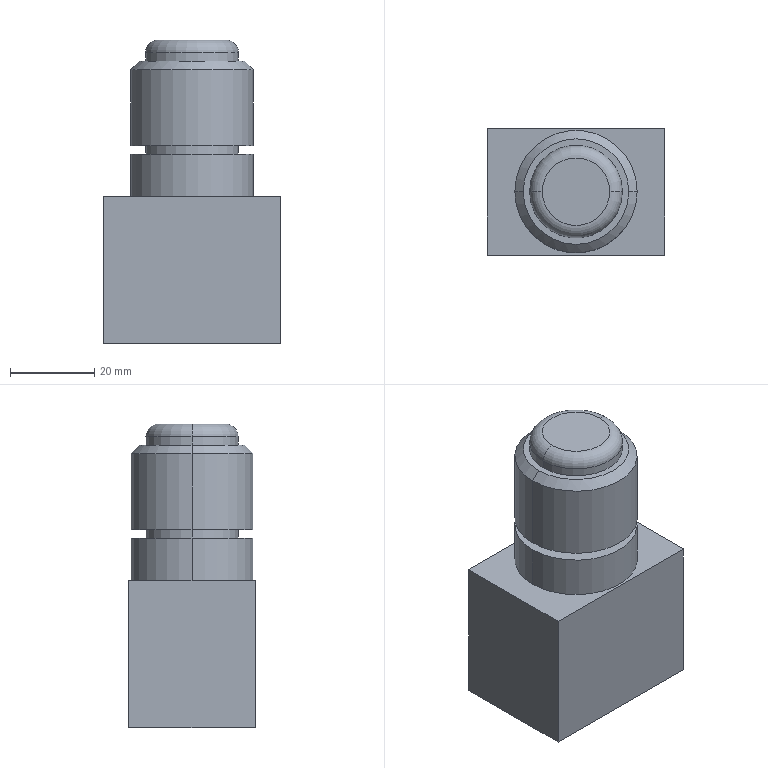Part | STEP file | Push button | 1 solid | 22 faces | box 42 x 30 x 72 mm | volume 66277 mm3 | plane 10 | cylinder 8 | cone 2 | torus 2 | commonest cylinder face diameters 22 x4 29 x4
STEP:
#1=CARTESIAN_POINT('',(0.,0.,0.));
#2=DIRECTION('',(0.,0.,1.));
#3=DIRECTION('',(1.,0.,0.));
#4=AXIS2_PLACEMENT_3D('',#1,#2,#3);
#5=CARTESIAN_POINT('',(12.5,0.,67.));
#6=VERTEX_POINT('',#5);
#7=CARTESIAN_POINT('',(-12.5,0.,67.));
#8=VERTEX_POINT('',#7);
#9=CARTESIAN_POINT('',(0.,0.,67.));
#10=DIRECTION('',(0.,0.,1.));
#11=DIRECTION('',(1.,0.,0.));
#12=AXIS2_PLACEMENT_3D('',#9,#10,#11);
#13=CIRCLE('',#12,12.5);
#14=CARTESIAN_POINT('',(0.,0.,67.));
#15=DIRECTION('',(0.,0.,-1.));
#16=DIRECTION('',(-1.,0.,0.));
#17=AXIS2_PLACEMENT_3D('',#14,#15,#16);
#18=CONICAL_SURFACE('',#17,12.5,0.7854);
#19=CARTESIAN_POINT('',(3.142,0.));
#20=DIRECTION('',(-1.,0.));
#21=VECTOR('',#20,1.);
#22=LINE('',#19,#21);
#23=(GEOMETRIC_REPRESENTATION_CONTEXT(2)PARAMETRIC_REPRESENTATION_CONTEXT()REPRESENTATION_CONTEXT('',''));
#24=DEFINITIONAL_REPRESENTATION('',(#22),#23);
#25=PCURVE('',#18,#24);
#26=CARTESIAN_POINT('',(0.,0.,67.));
#27=DIRECTION('',(0.,0.,1.));
#28=DIRECTION('',(1.,0.,0.));
#29=AXIS2_PLACEMENT_3D('',#26,#27,#28);
#30=PLANE('',#29);
#31=CARTESIAN_POINT('',(0.,0.));
#32=DIRECTION('',(1.,0.));
#33=AXIS2_PLACEMENT_2D('',#31,#32);
#34=CIRCLE('',#33,12.5);
#35=(GEOMETRIC_REPRESENTATION_CONTEXT(2)PARAMETRIC_REPRESENTATION_CONTEXT()REPRESENTATION_CONTEXT('',''));
#36=DEFINITIONAL_REPRESENTATION('',(#34),#35);
#37=PCURVE('',#30,#36);
#38=SURFACE_CURVE('',#13,(#25,#37),.PCURVE_S1.);
#39=EDGE_CURVE('',#6,#8,#38,.T.);
#40=ORIENTED_EDGE('',*,*,#39,.F.);
#41=CARTESIAN_POINT('',(14.5,0.,65.));
#42=VERTEX_POINT('',#41);
#43=CARTESIAN_POINT('',(12.5,0.,67.));
#44=DIRECTION('',(0.7071,0.,-0.7071));
#45=VECTOR('',#44,1.);
#46=LINE('',#43,#45);
#47=CARTESIAN_POINT('',(3.142,0.));
#48=DIRECTION('',(0.,1.));
#49=VECTOR('',#48,1.);
#50=LINE('',#47,#49);
#51=(GEOMETRIC_REPRESENTATION_CONTEXT(2)PARAMETRIC_REPRESENTATION_CONTEXT()REPRESENTATION_CONTEXT('',''));
#52=DEFINITIONAL_REPRESENTATION('',(#50),#51);
#53=PCURVE('',#18,#52);
#54=CARTESIAN_POINT('',(0.,0.,67.));
#55=DIRECTION('',(0.,0.,-1.));
#56=DIRECTION('',(-1.,0.,0.));
#57=AXIS2_PLACEMENT_3D('',#54,#55,#56);
#58=CONICAL_SURFACE('',#57,12.5,0.7854);
#59=CARTESIAN_POINT('',(3.142,0.));
#60=DIRECTION('',(0.,1.));
#61=VECTOR('',#60,1.);
#62=LINE('',#59,#61);
#63=(GEOMETRIC_REPRESENTATION_CONTEXT(2)PARAMETRIC_REPRESENTATION_CONTEXT()REPRESENTATION_CONTEXT('',''));
#64=DEFINITIONAL_REPRESENTATION('',(#62),#63);
#65=PCURVE('',#58,#64);
#66=SURFACE_CURVE('',#46,(#53,#65),.PCURVE_S1.);
#67=EDGE_CURVE('',#6,#42,#66,.T.);
#68=ORIENTED_EDGE('',*,*,#67,.T.);
#69=CARTESIAN_POINT('',(-14.5,0.,65.));
#70=VERTEX_POINT('',#69);
#71=CARTESIAN_POINT('',(0.,0.,65.));
#72=DIRECTION('',(0.,0.,-1.));
#73=DIRECTION('',(1.,0.,0.));
#74=AXIS2_PLACEMENT_3D('',#71,#72,#73);
#75=CIRCLE('',#74,14.5);
#76=CARTESIAN_POINT('',(-3.142,2.));
#77=DIRECTION('',(1.,0.));
#78=VECTOR('',#77,1.);
#79=LINE('',#76,#78);
#80=(GEOMETRIC_REPRESENTATION_CONTEXT(2)PARAMETRIC_REPRESENTATION_CONTEXT()REPRESENTATION_CONTEXT('',''));
#81=DEFINITIONAL_REPRESENTATION('',(#79),#80);
#82=PCURVE('',#18,#81);
#83=CARTESIAN_POINT('',(0.,0.,67.));
#84=DIRECTION('',(0.,0.,-1.));
#85=DIRECTION('',(-1.,0.,0.));
#86=AXIS2_PLACEMENT_3D('',#83,#84,#85);
#87=CYLINDRICAL_SURFACE('',#86,14.5);
#88=CARTESIAN_POINT('',(-3.142,2.));
#89=DIRECTION('',(1.,0.));
#90=VECTOR('',#89,1.);
#91=LINE('',#88,#90);
#92=(GEOMETRIC_REPRESENTATION_CONTEXT(2)PARAMETRIC_REPRESENTATION_CONTEXT()REPRESENTATION_CONTEXT('',''));
#93=DEFINITIONAL_REPRESENTATION('',(#91),#92);
#94=PCURVE('',#87,#93);
#95=SURFACE_CURVE('',#75,(#82,#94),.PCURVE_S1.);
#96=EDGE_CURVE('',#70,#42,#95,.T.);
#97=ORIENTED_EDGE('',*,*,#96,.F.);
#98=CARTESIAN_POINT('',(-12.5,0.,67.));
#99=DIRECTION('',(-0.7071,0.,-0.7071));
#100=VECTOR('',#99,1.);
#101=LINE('',#98,#100);
#102=CARTESIAN_POINT('',(0.,0.));
#103=DIRECTION('',(0.,1.));
#104=VECTOR('',#103,1.);
#105=LINE('',#102,#104);
#106=(GEOMETRIC_REPRESENTATION_CONTEXT(2)PARAMETRIC_REPRESENTATION_CONTEXT()REPRESENTATION_CONTEXT('',''));
#107=DEFINITIONAL_REPRESENTATION('',(#105),#106);
#108=PCURVE('',#18,#107);
#109=CARTESIAN_POINT('',(6.283,0.));
#110=DIRECTION('',(0.,1.));
#111=VECTOR('',#110,1.);
#112=LINE('',#109,#111);
#113=(GEOMETRIC_REPRESENTATION_CONTEXT(2)PARAMETRIC_REPRESENTATION_CONTEXT()REPRESENTATION_CONTEXT('',''));
#114=DEFINITIONAL_REPRESENTATION('',(#112),#113);
#115=PCURVE('',#58,#114);
#116=SURFACE_CURVE('',#101,(#108,#115),.PCURVE_S1.);
#117=EDGE_CURVE('',#8,#70,#116,.T.);
#118=ORIENTED_EDGE('',*,*,#117,.F.);
#119=EDGE_LOOP('',(#40,#68,#97,#118));
#120=FACE_BOUND('',#119,.T.);
#121=ADVANCED_FACE('',(#120),#18,.T.);
#122=CARTESIAN_POINT('',(-11.,0.,69.));
#123=VERTEX_POINT('',#122);
#124=CARTESIAN_POINT('',(11.,0.,69.));
#125=VERTEX_POINT('',#124);
#126=CARTESIAN_POINT('',(0.,0.,69.));
#127=DIRECTION('',(0.,0.,-1.));
#128=DIRECTION('',(1.,0.,0.));
#129=AXIS2_PLACEMENT_3D('',#126,#127,#128);
#130=CIRCLE('',#129,11.);
#131=CARTESIAN_POINT('',(0.,0.,69.));
#132=DIRECTION('',(0.,0.,1.));
#133=DIRECTION('',(1.,0.,0.));
#134=AXIS2_PLACEMENT_3D('',#131,#132,#133);
#135=TOROIDAL_SURFACE('',#134,8.,3.);
#136=CARTESIAN_POINT('',(6.283,0.));
#137=DIRECTION('',(-1.,0.));
#138=VECTOR('',#137,1.);
#139=LINE('',#136,#138);
#140=(GEOMETRIC_REPRESENTATION_CONTEXT(2)PARAMETRIC_REPRESENTATION_CONTEXT()REPRESENTATION_CONTEXT('',''));
#141=DEFINITIONAL_REPRESENTATION('',(#139),#140);
#142=PCURVE('',#135,#141);
#143=CARTESIAN_POINT('',(0.,0.,72.));
#144=DIRECTION('',(0.,0.,-1.));
#145=DIRECTION('',(-1.,0.,0.));
#146=AXIS2_PLACEMENT_3D('',#143,#144,#145);
#147=CYLINDRICAL_SURFACE('',#146,11.);
#148=CARTESIAN_POINT('',(-3.142,3.));
#149=DIRECTION('',(1.,0.));
#150=VECTOR('',#149,1.);
#151=LINE('',#148,#150);
#152=(GEOMETRIC_REPRESENTATION_CONTEXT(2)PARAMETRIC_REPRESENTATION_CONTEXT()REPRESENTATION_CONTEXT('',''));
#153=DEFINITIONAL_REPRESENTATION('',(#151),#152);
#154=PCURVE('',#147,#153);
#155=SURFACE_CURVE('',#130,(#142,#154),.PCURVE_S1.);
#156=EDGE_CURVE('',#123,#125,#155,.T.);
#157=ORIENTED_EDGE('',*,*,#156,.F.);
#158=CARTESIAN_POINT('',(-8.,0.,72.));
#159=VERTEX_POINT('',#158);
#160=CARTESIAN_POINT('',(-8.,0.,69.));
#161=DIRECTION('',(0.,1.,0.));
#162=DIRECTION('',(-1.,0.,0.));
#163=AXIS2_PLACEMENT_3D('',#160,#161,#162);
#164=CIRCLE('',#163,3.);
#165=CARTESIAN_POINT('',(3.142,0.));
#166=DIRECTION('',(0.,1.));
#167=VECTOR('',#166,1.);
#168=LINE('',#165,#167);
#169=(GEOMETRIC_REPRESENTATION_CONTEXT(2)PARAMETRIC_REPRESENTATION_CONTEXT()REPRESENTATION_CONTEXT('',''));
#170=DEFINITIONAL_REPRESENTATION('',(#168),#169);
#171=PCURVE('',#135,#170);
#172=CARTESIAN_POINT('',(0.,0.,69.));
#173=DIRECTION('',(0.,0.,1.));
#174=DIRECTION('',(1.,0.,0.));
#175=AXIS2_PLACEMENT_3D('',#172,#173,#174);
#176=TOROIDAL_SURFACE('',#175,8.,3.);
#177=CARTESIAN_POINT('',(3.142,0.));
#178=DIRECTION('',(0.,1.));
#179=VECTOR('',#178,1.);
#180=LINE('',#177,#179);
#181=(GEOMETRIC_REPRESENTATION_CONTEXT(2)PARAMETRIC_REPRESENTATION_CONTEXT()REPRESENTATION_CONTEXT('',''));
#182=DEFINITIONAL_REPRESENTATION('',(#180),#181);
#183=PCURVE('',#176,#182);
#184=SURFACE_CURVE('',#164,(#171,#183),.PCURVE_S1.);
#185=EDGE_CURVE('',#123,#159,#184,.T.);
#186=ORIENTED_EDGE('',*,*,#185,.T.);
#187=CARTESIAN_POINT('',(8.,0.,72.));
#188=VERTEX_POINT('',#187);
#189=CARTESIAN_POINT('',(0.,0.,72.));
#190=DIRECTION('',(0.,0.,1.));
#191=DIRECTION('',(1.,0.,0.));
#192=AXIS2_PLACEMENT_3D('',#189,#190,#191);
#193=CIRCLE('',#192,8.);
#194=CARTESIAN_POINT('',(0.,1.571));
#195=DIRECTION('',(1.,0.));
#196=VECTOR('',#195,1.);
#197=LINE('',#194,#196);
#198=(GEOMETRIC_REPRESENTATION_CONTEXT(2)PARAMETRIC_REPRESENTATION_CONTEXT()REPRESENTATION_CONTEXT('',''));
#199=DEFINITIONAL_REPRESENTATION('',(#197),#198);
#200=PCURVE('',#135,#199);
#201=CARTESIAN_POINT('',(0.,0.,72.));
#202=DIRECTION('',(0.,0.,1.));
#203=DIRECTION('',(1.,0.,0.));
#204=AXIS2_PLACEMENT_3D('',#201,#202,#203);
#205=PLANE('',#204);
#206=CARTESIAN_POINT('',(0.,0.));
#207=DIRECTION('',(1.,0.));
#208=AXIS2_PLACEMENT_2D('',#206,#207);
#209=CIRCLE('',#208,8.);
#210=(GEOMETRIC_REPRESENTATION_CONTEXT(2)PARAMETRIC_REPRESENTATION_CONTEXT()REPRESENTATION_CONTEXT('',''));
#211=DEFINITIONAL_REPRESENTATION('',(#209),#210);
#212=PCURVE('',#205,#211);
#213=SURFACE_CURVE('',#193,(#200,#212),.PCURVE_S1.);
#214=EDGE_CURVE('',#188,#159,#213,.T.);
#215=ORIENTED_EDGE('',*,*,#214,.F.);
#216=CARTESIAN_POINT('',(8.,0.,69.));
#217=DIRECTION('',(0.,-1.,0.));
#218=DIRECTION('',(0.,0.,-1.));
#219=AXIS2_PLACEMENT_3D('',#216,#217,#218);
#220=CIRCLE('',#219,3.);
#221=CARTESIAN_POINT('',(0.,-1.571));
#222=DIRECTION('',(0.,1.));
#223=VECTOR('',#222,1.);
#224=LINE('',#221,#223);
#225=(GEOMETRIC_REPRESENTATION_CONTEXT(2)PARAMETRIC_REPRESENTATION_CONTEXT()REPRESENTATION_CONTEXT('',''));
#226=DEFINITIONAL_REPRESENTATION('',(#224),#225);
#227=PCURVE('',#135,#226);
#228=CARTESIAN_POINT('',(6.283,-1.571));
#229=DIRECTION('',(0.,1.));
#230=VECTOR('',#229,1.);
#231=LINE('',#228,#230);
#232=(GEOMETRIC_REPRESENTATION_CONTEXT(2)PARAMETRIC_REPRESENTATION_CONTEXT()REPRESENTATION_CONTEXT('',''));
#233=DEFINITIONAL_REPRESENTATION('',(#231),#232);
#234=PCURVE('',#176,#233);
#235=SURFACE_CURVE('',#220,(#227,#234),.PCURVE_S1.);
#236=EDGE_CURVE('',#125,#188,#235,.T.);
#237=ORIENTED_EDGE('',*,*,#236,.F.);
#238=EDGE_LOOP('',(#157,#186,#215,#237));
#239=FACE_BOUND('',#238,.T.);
#240=ADVANCED_FACE('',(#239),#135,.T.);
#241=ORIENTED_EDGE('',*,*,#156,.T.);
#242=CARTESIAN_POINT('',(11.,0.,67.));
#243=VERTEX_POINT('',#242);
#244=CARTESIAN_POINT('',(11.,0.,72.));
#245=DIRECTION('',(0.,0.,-1.));
#246=VECTOR('',#245,1.);
#247=LINE('',#244,#246);
#248=CARTESIAN_POINT('',(3.142,0.));
#249=DIRECTION('',(0.,1.));
#250=VECTOR('',#249,1.);
#251=LINE('',#248,#250);
#252=(GEOMETRIC_REPRESENTATION_CONTEXT(2)PARAMETRIC_REPRESENTATION_CONTEXT()REPRESENTATION_CONTEXT('',''));
#253=DEFINITIONAL_REPRESENTATION('',(#251),#252);
#254=PCURVE('',#147,#253);
#255=CARTESIAN_POINT('',(0.,0.,72.));
#256=DIRECTION('',(0.,0.,-1.));
#257=DIRECTION('',(-1.,0.,0.));
#258=AXIS2_PLACEMENT_3D('',#255,#256,#257);
#259=CYLINDRICAL_SURFACE('',#258,11.);
#260=CARTESIAN_POINT('',(3.142,0.));
#261=DIRECTION('',(0.,1.));
#262=VECTOR('',#261,1.);
#263=LINE('',#260,#262);
#264=(GEOMETRIC_REPRESENTATION_CONTEXT(2)PARAMETRIC_REPRESENTATION_CONTEXT()REPRESENTATION_CONTEXT('',''));
#265=DEFINITIONAL_REPRESENTATION('',(#263),#264);
#266=PCURVE('',#259,#265);
#267=SURFACE_CURVE('',#247,(#254,#266),.PCURVE_S1.);
#268=EDGE_CURVE('',#125,#243,#267,.T.);
#269=ORIENTED_EDGE('',*,*,#268,.T.);
#270=CARTESIAN_POINT('',(-11.,0.,67.));
#271=VERTEX_POINT('',#270);
#272=CARTESIAN_POINT('',(0.,0.,67.));
#273=DIRECTION('',(0.,0.,1.));
#274=DIRECTION('',(1.,0.,0.));
#275=AXIS2_PLACEMENT_3D('',#272,#273,#274);
#276=CIRCLE('',#275,11.);
#277=CARTESIAN_POINT('',(3.142,5.));
#278=DIRECTION('',(-1.,0.));
#279=VECTOR('',#278,1.);
#280=LINE('',#277,#279);
#281=(GEOMETRIC_REPRESENTATION_CONTEXT(2)PARAMETRIC_REPRESENTATION_CONTEXT()REPRESENTATION_CONTEXT('',''));
#282=DEFINITIONAL_REPRESENTATION('',(#280),#281);
#283=PCURVE('',#147,#282);
#284=CARTESIAN_POINT('',(0.,0.));
#285=DIRECTION('',(1.,0.));
#286=AXIS2_PLACEMENT_2D('',#284,#285);
#287=CIRCLE('',#286,11.);
#288=(GEOMETRIC_REPRESENTATION_CONTEXT(2)PARAMETRIC_REPRESENTATION_CONTEXT()REPRESENTATION_CONTEXT('',''));
#289=DEFINITIONAL_REPRESENTATION('',(#287),#288);
#290=PCURVE('',#30,#289);
#291=SURFACE_CURVE('',#276,(#283,#290),.PCURVE_S1.);
#292=EDGE_CURVE('',#243,#271,#291,.T.);
#293=ORIENTED_EDGE('',*,*,#292,.T.);
#294=CARTESIAN_POINT('',(-11.,0.,72.));
#295=DIRECTION('',(0.,0.,-1.));
#296=VECTOR('',#295,1.);
#297=LINE('',#294,#296);
#298=CARTESIAN_POINT('',(0.,0.));
#299=DIRECTION('',(0.,1.));
#300=VECTOR('',#299,1.);
#301=LINE('',#298,#300);
#302=(GEOMETRIC_REPRESENTATION_CONTEXT(2)PARAMETRIC_REPRESENTATION_CONTEXT()REPRESENTATION_CONTEXT('',''));
#303=DEFINITIONAL_REPRESENTATION('',(#301),#302);
#304=PCURVE('',#147,#303);
#305=CARTESIAN_POINT('',(6.283,0.));
#306=DIRECTION('',(0.,1.));
#307=VECTOR('',#306,1.);
#308=LINE('',#305,#307);
#309=(GEOMETRIC_REPRESENTATION_CONTEXT(2)PARAMETRIC_REPRESENTATION_CONTEXT()REPRESENTATION_CONTEXT('',''));
#310=DEFINITIONAL_REPRESENTATION('',(#308),#309);
#311=PCURVE('',#259,#310);
#312=SURFACE_CURVE('',#297,(#304,#311),.PCURVE_S1.);
#313=EDGE_CURVE('',#123,#271,#312,.T.);
#314=ORIENTED_EDGE('',*,*,#313,.F.);
#315=EDGE_LOOP('',(#241,#269,#293,#314));
#316=FACE_BOUND('',#315,.T.);
#317=ADVANCED_FACE('',(#316),#147,.T.);
#318=ORIENTED_EDGE('',*,*,#96,.T.);
#319=CARTESIAN_POINT('',(14.5,0.,47.));
#320=VERTEX_POINT('',#319);
#321=CARTESIAN_POINT('',(14.5,0.,67.));
#322=DIRECTION('',(0.,0.,-1.));
#323=VECTOR('',#322,1.);
#324=LINE('',#321,#323);
#325=CARTESIAN_POINT('',(3.142,0.));
#326=DIRECTION('',(0.,1.));
#327=VECTOR('',#326,1.);
#328=LINE('',#325,#327);
#329=(GEOMETRIC_REPRESENTATION_CONTEXT(2)PARAMETRIC_REPRESENTATION_CONTEXT()REPRESENTATION_CONTEXT('',''));
#330=DEFINITIONAL_REPRESENTATION('',(#328),#329);
#331=PCURVE('',#87,#330);
#332=CARTESIAN_POINT('',(0.,0.,67.));
#333=DIRECTION('',(0.,0.,-1.));
#334=DIRECTION('',(-1.,0.,0.));
#335=AXIS2_PLACEMENT_3D('',#332,#333,#334);
#336=CYLINDRICAL_SURFACE('',#335,14.5);
#337=CARTESIAN_POINT('',(3.142,0.));
#338=DIRECTION('',(0.,1.));
#339=VECTOR('',#338,1.);
#340=LINE('',#337,#339);
#341=(GEOMETRIC_REPRESENTATION_CONTEXT(2)PARAMETRIC_REPRESENTATION_CONTEXT()REPRESENTATION_CONTEXT('',''));
#342=DEFINITIONAL_REPRESENTATION('',(#340),#341);
#343=PCURVE('',#336,#342);
#344=SURFACE_CURVE('',#324,(#331,#343),.PCURVE_S1.);
#345=EDGE_CURVE('',#42,#320,#344,.T.);
#346=ORIENTED_EDGE('',*,*,#345,.T.);
#347=CARTESIAN_POINT('',(-14.5,0.,47.));
#348=VERTEX_POINT('',#347);
#349=CARTESIAN_POINT('',(0.,0.,47.));
#350=DIRECTION('',(0.,0.,1.));
#351=DIRECTION('',(1.,0.,0.));
#352=AXIS2_PLACEMENT_3D('',#349,#350,#351);
#353=CIRCLE('',#352,14.5);
#354=CARTESIAN_POINT('',(3.142,20.));
#355=DIRECTION('',(-1.,0.));
#356=VECTOR('',#355,1.);
#357=LINE('',#354,#356);
#358=(GEOMETRIC_REPRESENTATION_CONTEXT(2)PARAMETRIC_REPRESENTATION_CONTEXT()REPRESENTATION_CONTEXT('',''));
#359=DEFINITIONAL_REPRESENTATION('',(#357),#358);
#360=PCURVE('',#87,#359);
#361=CARTESIAN_POINT('',(0.,0.,47.));
#362=DIRECTION('',(0.,0.,1.));
#363=DIRECTION('',(1.,0.,0.));
#364=AXIS2_PLACEMENT_3D('',#361,#362,#363);
#365=PLANE('',#364);
#366=CARTESIAN_POINT('',(0.,0.));
#367=DIRECTION('',(1.,0.));
#368=AXIS2_PLACEMENT_2D('',#366,#367);
#369=CIRCLE('',#368,14.5);
#370=(GEOMETRIC_REPRESENTATION_CONTEXT(2)PARAMETRIC_REPRESENTATION_CONTEXT()REPRESENTATION_CONTEXT('',''));
#371=DEFINITIONAL_REPRESENTATION('',(#369),#370);
#372=PCURVE('',#365,#371);
#373=SURFACE_CURVE('',#353,(#360,#372),.PCURVE_S1.);
#374=EDGE_CURVE('',#320,#348,#373,.T.);
#375=ORIENTED_EDGE('',*,*,#374,.T.);
#376=CARTESIAN_POINT('',(-14.5,0.,67.));
#377=DIRECTION('',(0.,0.,-1.));
#378=VECTOR('',#377,1.);
#379=LINE('',#376,#378);
#380=CARTESIAN_POINT('',(0.,0.));
#381=DIRECTION('',(0.,1.));
#382=VECTOR('',#381,1.);
#383=LINE('',#380,#382);
#384=(GEOMETRIC_REPRESENTATION_CONTEXT(2)PARAMETRIC_REPRESENTATION_CONTEXT()REPRESENTATION_CONTEXT('',''));
#385=DEFINITIONAL_REPRESENTATION('',(#383),#384);
#386=PCURVE('',#87,#385);
#387=CARTESIAN_POINT('',(6.283,0.));
#388=DIRECTION('',(0.,1.));
#389=VECTOR('',#388,1.);
#390=LINE('',#387,#389);
#391=(GEOMETRIC_REPRESENTATION_CONTEXT(2)PARAMETRIC_REPRESENTATION_CONTEXT()REPRESENTATION_CONTEXT('',''));
#392=DEFINITIONAL_REPRESENTATION('',(#390),#391);
#393=PCURVE('',#336,#392);
#394=SURFACE_CURVE('',#379,(#386,#393),.PCURVE_S1.);
#395=EDGE_CURVE('',#70,#348,#394,.T.);
#396=ORIENTED_EDGE('',*,*,#395,.F.);
#397=EDGE_LOOP('',(#318,#346,#375,#396));
#398=FACE_BOUND('',#397,.T.);
#399=ADVANCED_FACE('',(#398),#87,.T.);
#400=CARTESIAN_POINT('',(11.,0.,47.));
#401=VERTEX_POINT('',#400);
#402=CARTESIAN_POINT('',(-11.,0.,47.));
#403=VERTEX_POINT('',#402);
#404=CARTESIAN_POINT('',(0.,0.,47.));
#405=DIRECTION('',(0.,0.,1.));
#406=DIRECTION('',(1.,0.,0.));
#407=AXIS2_PLACEMENT_3D('',#404,#405,#406);
#408=CIRCLE('',#407,11.);
#409=CARTESIAN_POINT('',(0.,0.,47.));
#410=DIRECTION('',(0.,0.,-1.));
#411=DIRECTION('',(-1.,0.,0.));
#412=AXIS2_PLACEMENT_3D('',#409,#410,#411);
#413=CYLINDRICAL_SURFACE('',#412,11.);
#414=CARTESIAN_POINT('',(3.142,0.));
#415=DIRECTION('',(-1.,0.));
#416=VECTOR('',#415,1.);
#417=LINE('',#414,#416);
#418=(GEOMETRIC_REPRESENTATION_CONTEXT(2)PARAMETRIC_REPRESENTATION_CONTEXT()REPRESENTATION_CONTEXT('',''));
#419=DEFINITIONAL_REPRESENTATION('',(#417),#418);
#420=PCURVE('',#413,#419);
#421=CARTESIAN_POINT('',(0.,0.));
#422=DIRECTION('',(1.,0.));
#423=AXIS2_PLACEMENT_2D('',#421,#422);
#424=CIRCLE('',#423,11.);
#425=(GEOMETRIC_REPRESENTATION_CONTEXT(2)PARAMETRIC_REPRESENTATION_CONTEXT()REPRESENTATION_CONTEXT('',''));
#426=DEFINITIONAL_REPRESENTATION('',(#424),#425);
#427=PCURVE('',#365,#426);
#428=SURFACE_CURVE('',#408,(#420,#427),.PCURVE_S1.);
#429=EDGE_CURVE('',#401,#403,#428,.T.);
#430=ORIENTED_EDGE('',*,*,#429,.F.);
#431=CARTESIAN_POINT('',(11.,0.,45.));
#432=VERTEX_POINT('',#431);
#433=CARTESIAN_POINT('',(11.,0.,47.));
#434=DIRECTION('',(0.,0.,-1.));
#435=VECTOR('',#434,1.);
#436=LINE('',#433,#435);
#437=CARTESIAN_POINT('',(3.142,0.));
#438=DIRECTION('',(0.,1.));
#439=VECTOR('',#438,1.);
#440=LINE('',#437,#439);
#441=(GEOMETRIC_REPRESENTATION_CONTEXT(2)PARAMETRIC_REPRESENTATION_CONTEXT()REPRESENTATION_CONTEXT('',''));
#442=DEFINITIONAL_REPRESENTATION('',(#440),#441);
#443=PCURVE('',#413,#442);
#444=CARTESIAN_POINT('',(0.,0.,47.));
#445=DIRECTION('',(0.,0.,-1.));
#446=DIRECTION('',(-1.,0.,0.));
#447=AXIS2_PLACEMENT_3D('',#444,#445,#446);
#448=CYLINDRICAL_SURFACE('',#447,11.);
#449=CARTESIAN_POINT('',(3.142,0.));
#450=DIRECTION('',(0.,1.));
#451=VECTOR('',#450,1.);
#452=LINE('',#449,#451);
#453=(GEOMETRIC_REPRESENTATION_CONTEXT(2)PARAMETRIC_REPRESENTATION_CONTEXT()REPRESENTATION_CONTEXT('',''));
#454=DEFINITIONAL_REPRESENTATION('',(#452),#453);
#455=PCURVE('',#448,#454);
#456=SURFACE_CURVE('',#436,(#443,#455),.PCURVE_S1.);
#457=EDGE_CURVE('',#401,#432,#456,.T.);
#458=ORIENTED_EDGE('',*,*,#457,.T.);
#459=CARTESIAN_POINT('',(-11.,0.,45.));
#460=VERTEX_POINT('',#459);
#461=CARTESIAN_POINT('',(0.,0.,45.));
#462=DIRECTION('',(0.,0.,1.));
#463=DIRECTION('',(1.,0.,0.));
#464=AXIS2_PLACEMENT_3D('',#461,#462,#463);
#465=CIRCLE('',#464,11.);
#466=CARTESIAN_POINT('',(3.142,2.));
#467=DIRECTION('',(-1.,0.));
#468=VECTOR('',#467,1.);
#469=LINE('',#466,#468);
#470=(GEOMETRIC_REPRESENTATION_CONTEXT(2)PARAMETRIC_REPRESENTATION_CONTEXT()REPRESENTATION_CONTEXT('',''));
#471=DEFINITIONAL_REPRESENTATION('',(#469),#470);
#472=PCURVE('',#413,#471);
#473=CARTESIAN_POINT('',(0.,0.,45.));
#474=DIRECTION('',(0.,0.,1.));
#475=DIRECTION('',(1.,0.,0.));
#476=AXIS2_PLACEMENT_3D('',#473,#474,#475);
#477=PLANE('',#476);
#478=CARTESIAN_POINT('',(0.,0.));
#479=DIRECTION('',(1.,0.));
#480=AXIS2_PLACEMENT_2D('',#478,#479);
#481=CIRCLE('',#480,11.);
#482=(GEOMETRIC_REPRESENTATION_CONTEXT(2)PARAMETRIC_REPRESENTATION_CONTEXT()REPRESENTATION_CONTEXT('',''));
#483=DEFINITIONAL_REPRESENTATION('',(#481),#482);
#484=PCURVE('',#477,#483);
#485=SURFACE_CURVE('',#465,(#472,#484),.PCURVE_S1.);
#486=EDGE_CURVE('',#432,#460,#485,.T.);
#487=ORIENTED_EDGE('',*,*,#486,.T.);
#488=CARTESIAN_POINT('',(-11.,0.,47.));
#489=DIRECTION('',(0.,0.,-1.));
#490=VECTOR('',#489,1.);
#491=LINE('',#488,#490);
#492=CARTESIAN_POINT('',(0.,0.));
#493=DIRECTION('',(0.,1.));
#494=VECTOR('',#493,1.);
#495=LINE('',#492,#494);
#496=(GEOMETRIC_REPRESENTATION_CONTEXT(2)PARAMETRIC_REPRESENTATION_CONTEXT()REPRESENTATION_CONTEXT('',''));
#497=DEFINITIONAL_REPRESENTATION('',(#495),#496);
#498=PCURVE('',#413,#497);
#499=CARTESIAN_POINT('',(6.283,0.));
#500=DIRECTION('',(0.,1.));
#501=VECTOR('',#500,1.);
#502=LINE('',#499,#501);
#503=(GEOMETRIC_REPRESENTATION_CONTEXT(2)PARAMETRIC_REPRESENTATION_CONTEXT()REPRESENTATION_CONTEXT('',''));
#504=DEFINITIONAL_REPRESENTATION('',(#502),#503);
#505=PCURVE('',#448,#504);
#506=SURFACE_CURVE('',#491,(#498,#505),.PCURVE_S1.);
#507=EDGE_CURVE('',#403,#460,#506,.T.);
#508=ORIENTED_EDGE('',*,*,#507,.F.);
#509=EDGE_LOOP('',(#430,#458,#487,#508));
#510=FACE_BOUND('',#509,.T.);
#511=ADVANCED_FACE('',(#510),#413,.T.);
#512=CARTESIAN_POINT('',(14.5,0.,45.));
#513=VERTEX_POINT('',#512);
#514=CARTESIAN_POINT('',(-14.5,0.,45.));
#515=VERTEX_POINT('',#514);
#516=CARTESIAN_POINT('',(0.,0.,45.));
#517=DIRECTION('',(0.,0.,1.));
#518=DIRECTION('',(1.,0.,0.));
#519=AXIS2_PLACEMENT_3D('',#516,#517,#518);
#520=CIRCLE('',#519,14.5);
#521=CARTESIAN_POINT('',(0.,0.,45.));
#522=DIRECTION('',(0.,0.,-1.));
#523=DIRECTION('',(-1.,0.,0.));
#524=AXIS2_PLACEMENT_3D('',#521,#522,#523);
#525=CYLINDRICAL_SURFACE('',#524,14.5);
#526=CARTESIAN_POINT('',(3.142,0.));
#527=DIRECTION('',(-1.,0.));
#528=VECTOR('',#527,1.);
#529=LINE('',#526,#528);
#530=(GEOMETRIC_REPRESENTATION_CONTEXT(2)PARAMETRIC_REPRESENTATION_CONTEXT()REPRESENTATION_CONTEXT('',''));
#531=DEFINITIONAL_REPRESENTATION('',(#529),#530);
#532=PCURVE('',#525,#531);
#533=CARTESIAN_POINT('',(0.,0.));
#534=DIRECTION('',(1.,0.));
#535=AXIS2_PLACEMENT_2D('',#533,#534);
#536=CIRCLE('',#535,14.5);
#537=(GEOMETRIC_REPRESENTATION_CONTEXT(2)PARAMETRIC_REPRESENTATION_CONTEXT()REPRESENTATION_CONTEXT('',''));
#538=DEFINITIONAL_REPRESENTATION('',(#536),#537);
#539=PCURVE('',#477,#538);
#540=SURFACE_CURVE('',#520,(#532,#539),.PCURVE_S1.);
#541=EDGE_CURVE('',#513,#515,#540,.T.);
#542=ORIENTED_EDGE('',*,*,#541,.F.);
#543=CARTESIAN_POINT('',(14.5,0.,35.));
#544=VERTEX_POINT('',#543);
#545=CARTESIAN_POINT('',(14.5,0.,45.));
#546=DIRECTION('',(0.,0.,-1.));
#547=VECTOR('',#546,1.);
#548=LINE('',#545,#547);
#549=CARTESIAN_POINT('',(3.142,0.));
#550=DIRECTION('',(0.,1.));
#551=VECTOR('',#550,1.);
#552=LINE('',#549,#551);
#553=(GEOMETRIC_REPRESENTATION_CONTEXT(2)PARAMETRIC_REPRESENTATION_CONTEXT()REPRESENTATION_CONTEXT('',''));
#554=DEFINITIONAL_REPRESENTATION('',(#552),#553);
#555=PCURVE('',#525,#554);
#556=CARTESIAN_POINT('',(0.,0.,45.));
#557=DIRECTION('',(0.,0.,-1.));
#558=DIRECTION('',(-1.,0.,0.));
#559=AXIS2_PLACEMENT_3D('',#556,#557,#558);
#560=CYLINDRICAL_SURFACE('',#559,14.5);
#561=CARTESIAN_POINT('',(3.142,0.));
#562=DIRECTION('',(0.,1.));
#563=VECTOR('',#562,1.);
#564=LINE('',#561,#563);
#565=(GEOMETRIC_REPRESENTATION_CONTEXT(2)PARAMETRIC_REPRESENTATION_CONTEXT()REPRESENTATION_CONTEXT('',''));
#566=DEFINITIONAL_REPRESENTATION('',(#564),#565);
#567=PCURVE('',#560,#566);
#568=SURFACE_CURVE('',#548,(#555,#567),.PCURVE_S1.);
#569=EDGE_CURVE('',#513,#544,#568,.T.);
#570=ORIENTED_EDGE('',*,*,#569,.T.);
#571=CARTESIAN_POINT('',(-14.5,0.,35.));
#572=VERTEX_POINT('',#571);
#573=CARTESIAN_POINT('',(0.,0.,35.));
#574=DIRECTION('',(0.,0.,1.));
#575=DIRECTION('',(1.,0.,0.));
#576=AXIS2_PLACEMENT_3D('',#573,#574,#575);
#577=CIRCLE('',#576,14.5);
#578=CARTESIAN_POINT('',(3.142,10.));
#579=DIRECTION('',(-1.,0.));
#580=VECTOR('',#579,1.);
#581=LINE('',#578,#580);
#582=(GEOMETRIC_REPRESENTATION_CONTEXT(2)PARAMETRIC_REPRESENTATION_CONTEXT()REPRESENTATION_CONTEXT('',''));
#583=DEFINITIONAL_REPRESENTATION('',(#581),#582);
#584=PCURVE('',#525,#583);
#585=CARTESIAN_POINT('',(0.,0.,35.));
#586=DIRECTION('',(0.,0.,1.));
#587=DIRECTION('',(1.,0.,0.));
#588=AXIS2_PLACEMENT_3D('',#585,#586,#587);
#589=PLANE('',#588);
#590=CARTESIAN_POINT('',(0.,0.));
#591=DIRECTION('',(1.,0.));
#592=AXIS2_PLACEMENT_2D('',#590,#591);
#593=CIRCLE('',#592,14.5);
#594=(GEOMETRIC_REPRESENTATION_CONTEXT(2)PARAMETRIC_REPRESENTATION_CONTEXT()REPRESENTATION_CONTEXT('',''));
#595=DEFINITIONAL_REPRESENTATION('',(#593),#594);
#596=PCURVE('',#589,#595);
#597=SURFACE_CURVE('',#577,(#584,#596),.PCURVE_S1.);
#598=EDGE_CURVE('',#544,#572,#597,.T.);
#599=ORIENTED_EDGE('',*,*,#598,.T.);
#600=CARTESIAN_POINT('',(-14.5,0.,45.));
#601=DIRECTION('',(0.,0.,-1.));
#602=VECTOR('',#601,1.);
#603=LINE('',#600,#602);
#604=CARTESIAN_POINT('',(0.,0.));
#605=DIRECTION('',(0.,1.));
#606=VECTOR('',#605,1.);
#607=LINE('',#604,#606);
#608=(GEOMETRIC_REPRESENTATION_CONTEXT(2)PARAMETRIC_REPRESENTATION_CONTEXT()REPRESENTATION_CONTEXT('',''));
#609=DEFINITIONAL_REPRESENTATION('',(#607),#608);
#610=PCURVE('',#525,#609);
#611=CARTESIAN_POINT('',(6.283,0.));
#612=DIRECTION('',(0.,1.));
#613=VECTOR('',#612,1.);
#614=LINE('',#611,#613);
#615=(GEOMETRIC_REPRESENTATION_CONTEXT(2)PARAMETRIC_REPRESENTATION_CONTEXT()REPRESENTATION_CONTEXT('',''));
#616=DEFINITIONAL_REPRESENTATION('',(#614),#615);
#617=PCURVE('',#560,#616);
#618=SURFACE_CURVE('',#603,(#610,#617),.PCURVE_S1.);
#619=EDGE_CURVE('',#515,#572,#618,.T.);
#620=ORIENTED_EDGE('',*,*,#619,.F.);
#621=EDGE_LOOP('',(#542,#570,#599,#620));
#622=FACE_BOUND('',#621,.T.);
#623=ADVANCED_FACE('',(#622),#525,.T.);
#624=CARTESIAN_POINT('',(0.,0.,67.));
#625=DIRECTION('',(0.,0.,1.));
#626=DIRECTION('',(1.,0.,0.));
#627=AXIS2_PLACEMENT_3D('',#624,#625,#626);
#628=CIRCLE('',#627,12.5);
#629=CARTESIAN_POINT('',(0.,0.));
#630=DIRECTION('',(1.,0.));
#631=AXIS2_PLACEMENT_2D('',#629,#630);
#632=CIRCLE('',#631,12.5);
#633=(GEOMETRIC_REPRESENTATION_CONTEXT(2)PARAMETRIC_REPRESENTATION_CONTEXT()REPRESENTATION_CONTEXT('',''));
#634=DEFINITIONAL_REPRESENTATION('',(#632),#633);
#635=PCURVE('',#30,#634);
#636=CARTESIAN_POINT('',(9.425,0.));
#637=DIRECTION('',(-1.,0.));
#638=VECTOR('',#637,1.);
#639=LINE('',#636,#638);
#640=(GEOMETRIC_REPRESENTATION_CONTEXT(2)PARAMETRIC_REPRESENTATION_CONTEXT()REPRESENTATION_CONTEXT('',''));
#641=DEFINITIONAL_REPRESENTATION('',(#639),#640);
#642=PCURVE('',#58,#641);
#643=SURFACE_CURVE('',#628,(#635,#642),.PCURVE_S1.);
#644=EDGE_CURVE('',#8,#6,#643,.T.);
#645=ORIENTED_EDGE('',*,*,#644,.T.);
#646=ORIENTED_EDGE('',*,*,#39,.T.);
#647=EDGE_LOOP('',(#645,#646));
#648=FACE_BOUND('',#647,.T.);
#649=CARTESIAN_POINT('',(0.,0.,67.));
#650=DIRECTION('',(0.,0.,1.));
#651=DIRECTION('',(1.,0.,0.));
#652=AXIS2_PLACEMENT_3D('',#649,#650,#651);
#653=CIRCLE('',#652,11.);
#654=CARTESIAN_POINT('',(0.,0.));
#655=DIRECTION('',(1.,0.));
#656=AXIS2_PLACEMENT_2D('',#654,#655);
#657=CIRCLE('',#656,11.);
#658=(GEOMETRIC_REPRESENTATION_CONTEXT(2)PARAMETRIC_REPRESENTATION_CONTEXT()REPRESENTATION_CONTEXT('',''));
#659=DEFINITIONAL_REPRESENTATION('',(#657),#658);
#660=PCURVE('',#30,#659);
#661=CARTESIAN_POINT('',(9.425,5.));
#662=DIRECTION('',(-1.,0.));
#663=VECTOR('',#662,1.);
#664=LINE('',#661,#663);
#665=(GEOMETRIC_REPRESENTATION_CONTEXT(2)PARAMETRIC_REPRESENTATION_CONTEXT()REPRESENTATION_CONTEXT('',''));
#666=DEFINITIONAL_REPRESENTATION('',(#664),#665);
#667=PCURVE('',#259,#666);
#668=SURFACE_CURVE('',#653,(#660,#667),.PCURVE_S1.);
#669=EDGE_CURVE('',#271,#243,#668,.T.);
#670=ORIENTED_EDGE('',*,*,#669,.F.);
#671=ORIENTED_EDGE('',*,*,#292,.F.);
#672=EDGE_LOOP('',(#670,#671));
#673=FACE_BOUND('',#672,.T.);
#674=ADVANCED_FACE('',(#648,#673),#30,.T.);
#675=CARTESIAN_POINT('',(0.,0.,45.));
#676=DIRECTION('',(0.,0.,1.));
#677=DIRECTION('',(1.,0.,0.));
#678=AXIS2_PLACEMENT_3D('',#675,#676,#677);
#679=CIRCLE('',#678,14.5);
#680=CARTESIAN_POINT('',(0.,0.));
#681=DIRECTION('',(1.,0.));
#682=AXIS2_PLACEMENT_2D('',#680,#681);
#683=CIRCLE('',#682,14.5);
#684=(GEOMETRIC_REPRESENTATION_CONTEXT(2)PARAMETRIC_REPRESENTATION_CONTEXT()REPRESENTATION_CONTEXT('',''));
#685=DEFINITIONAL_REPRESENTATION('',(#683),#684);
#686=PCURVE('',#477,#685);
#687=CARTESIAN_POINT('',(9.425,0.));
#688=DIRECTION('',(-1.,0.));
#689=VECTOR('',#688,1.);
#690=LINE('',#687,#689);
#691=(GEOMETRIC_REPRESENTATION_CONTEXT(2)PARAMETRIC_REPRESENTATION_CONTEXT()REPRESENTATION_CONTEXT('',''));
#692=DEFINITIONAL_REPRESENTATION('',(#690),#691);
#693=PCURVE('',#560,#692);
#694=SURFACE_CURVE('',#679,(#686,#693),.PCURVE_S1.);
#695=EDGE_CURVE('',#515,#513,#694,.T.);
#696=ORIENTED_EDGE('',*,*,#695,.T.);
#697=ORIENTED_EDGE('',*,*,#541,.T.);
#698=EDGE_LOOP('',(#696,#697));
#699=FACE_BOUND('',#698,.T.);
#700=CARTESIAN_POINT('',(0.,0.,45.));
#701=DIRECTION('',(0.,0.,1.));
#702=DIRECTION('',(1.,0.,0.));
#703=AXIS2_PLACEMENT_3D('',#700,#701,#702);
#704=CIRCLE('',#703,11.);
#705=CARTESIAN_POINT('',(0.,0.));
#706=DIRECTION('',(1.,0.));
#707=AXIS2_PLACEMENT_2D('',#705,#706);
#708=CIRCLE('',#707,11.);
#709=(GEOMETRIC_REPRESENTATION_CONTEXT(2)PARAMETRIC_REPRESENTATION_CONTEXT()REPRESENTATION_CONTEXT('',''));
#710=DEFINITIONAL_REPRESENTATION('',(#708),#709);
#711=PCURVE('',#477,#710);
#712=CARTESIAN_POINT('',(9.425,2.));
#713=DIRECTION('',(-1.,0.));
#714=VECTOR('',#713,1.);
#715=LINE('',#712,#714);
#716=(GEOMETRIC_REPRESENTATION_CONTEXT(2)PARAMETRIC_REPRESENTATION_CONTEXT()REPRESENTATION_CONTEXT('',''));
#717=DEFINITIONAL_REPRESENTATION('',(#715),#716);
#718=PCURVE('',#448,#717);
#719=SURFACE_CURVE('',#704,(#711,#718),.PCURVE_S1.);
#720=EDGE_CURVE('',#460,#432,#719,.T.);
#721=ORIENTED_EDGE('',*,*,#720,.F.);
#722=ORIENTED_EDGE('',*,*,#486,.F.);
#723=EDGE_LOOP('',(#721,#722));
#724=FACE_BOUND('',#723,.T.);
#725=ADVANCED_FACE('',(#699,#724),#477,.T.);
#726=CARTESIAN_POINT('',(21.,-15.,35.));
#727=VERTEX_POINT('',#726);
#728=CARTESIAN_POINT('',(21.,15.,35.));
#729=VERTEX_POINT('',#728);
#730=CARTESIAN_POINT('',(21.,15.,35.));
#731=DIRECTION('',(0.,1.,0.));
#732=VECTOR('',#731,1.);
#733=LINE('',#730,#732);
#734=CARTESIAN_POINT('',(21.,15.));
#735=DIRECTION('',(0.,1.));
#736=VECTOR('',#735,1.);
#737=LINE('',#734,#736);
#738=(GEOMETRIC_REPRESENTATION_CONTEXT(2)PARAMETRIC_REPRESENTATION_CONTEXT()REPRESENTATION_CONTEXT('',''));
#739=DEFINITIONAL_REPRESENTATION('',(#737),#738);
#740=PCURVE('',#589,#739);
#741=CARTESIAN_POINT('',(21.,15.,35.));
#742=DIRECTION('',(-1.,0.,0.));
#743=DIRECTION('',(0.,-1.,0.));
#744=AXIS2_PLACEMENT_3D('',#741,#742,#743);
#745=PLANE('',#744);
#746=CARTESIAN_POINT('',(0.,0.));
#747=DIRECTION('',(-1.,0.));
#748=VECTOR('',#747,1.);
#749=LINE('',#746,#748);
#750=(GEOMETRIC_REPRESENTATION_CONTEXT(2)PARAMETRIC_REPRESENTATION_CONTEXT()REPRESENTATION_CONTEXT('',''));
#751=DEFINITIONAL_REPRESENTATION('',(#749),#750);
#752=PCURVE('',#745,#751);
#753=SURFACE_CURVE('',#733,(#740,#752),.PCURVE_S1.);
#754=EDGE_CURVE('',#727,#729,#753,.T.);
#755=ORIENTED_EDGE('',*,*,#754,.T.);
#756=CARTESIAN_POINT('',(-21.,15.,35.));
#757=VERTEX_POINT('',#756);
#758=CARTESIAN_POINT('',(-21.,15.,35.));
#759=DIRECTION('',(-1.,0.,0.));
#760=VECTOR('',#759,1.);
#761=LINE('',#758,#760);
#762=CARTESIAN_POINT('',(-21.,15.));
#763=DIRECTION('',(-1.,0.));
#764=VECTOR('',#763,1.);
#765=LINE('',#762,#764);
#766=(GEOMETRIC_REPRESENTATION_CONTEXT(2)PARAMETRIC_REPRESENTATION_CONTEXT()REPRESENTATION_CONTEXT('',''));
#767=DEFINITIONAL_REPRESENTATION('',(#765),#766);
#768=PCURVE('',#589,#767);
#769=CARTESIAN_POINT('',(-21.,15.,35.));
#770=DIRECTION('',(0.,-1.,0.));
#771=DIRECTION('',(0.,0.,-1.));
#772=AXIS2_PLACEMENT_3D('',#769,#770,#771);
#773=PLANE('',#772);
#774=CARTESIAN_POINT('',(0.,0.));
#775=DIRECTION('',(0.,-1.));
#776=VECTOR('',#775,1.);
#777=LINE('',#774,#776);
#778=(GEOMETRIC_REPRESENTATION_CONTEXT(2)PARAMETRIC_REPRESENTATION_CONTEXT()REPRESENTATION_CONTEXT('',''));
#779=DEFINITIONAL_REPRESENTATION('',(#777),#778);
#780=PCURVE('',#773,#779);
#781=SURFACE_CURVE('',#761,(#768,#780),.PCURVE_S1.);
#782=EDGE_CURVE('',#729,#757,#781,.T.);
#783=ORIENTED_EDGE('',*,*,#782,.T.);
#784=CARTESIAN_POINT('',(-21.,-15.,35.));
#785=VERTEX_POINT('',#784);
#786=CARTESIAN_POINT('',(-21.,15.,35.));
#787=DIRECTION('',(0.,-1.,0.));
#788=VECTOR('',#787,1.);
#789=LINE('',#786,#788);
#790=CARTESIAN_POINT('',(-21.,15.));
#791=DIRECTION('',(0.,-1.));
#792=VECTOR('',#791,1.);
#793=LINE('',#790,#792);
#794=(GEOMETRIC_REPRESENTATION_CONTEXT(2)PARAMETRIC_REPRESENTATION_CONTEXT()REPRESENTATION_CONTEXT('',''));
#795=DEFINITIONAL_REPRESENTATION('',(#793),#794);
#796=PCURVE('',#589,#795);
#797=CARTESIAN_POINT('',(-21.,15.,35.));
#798=DIRECTION('',(1.,0.,0.));
#799=DIRECTION('',(0.,0.,-1.));
#800=AXIS2_PLACEMENT_3D('',#797,#798,#799);
#801=PLANE('',#800);
#802=CARTESIAN_POINT('',(0.,0.));
#803=DIRECTION('',(0.,-1.));
#804=VECTOR('',#803,1.);
#805=LINE('',#802,#804);
#806=(GEOMETRIC_REPRESENTATION_CONTEXT(2)PARAMETRIC_REPRESENTATION_CONTEXT()REPRESENTATION_CONTEXT('',''));
#807=DEFINITIONAL_REPRESENTATION('',(#805),#806);
#808=PCURVE('',#801,#807);
#809=SURFACE_CURVE('',#789,(#796,#808),.PCURVE_S1.);
#810=EDGE_CURVE('',#757,#785,#809,.T.);
#811=ORIENTED_EDGE('',*,*,#810,.T.);
#812=CARTESIAN_POINT('',(-21.,-15.,35.));
#813=DIRECTION('',(1.,0.,0.));
#814=VECTOR('',#813,1.);
#815=LINE('',#812,#814);
#816=CARTESIAN_POINT('',(-21.,-15.));
#817=DIRECTION('',(1.,0.));
#818=VECTOR('',#817,1.);
#819=LINE('',#816,#818);
#820=(GEOMETRIC_REPRESENTATION_CONTEXT(2)PARAMETRIC_REPRESENTATION_CONTEXT()REPRESENTATION_CONTEXT('',''));
#821=DEFINITIONAL_REPRESENTATION('',(#819),#820);
#822=PCURVE('',#589,#821);
#823=CARTESIAN_POINT('',(-21.,-15.,35.));
#824=DIRECTION('',(0.,1.,0.));
#825=DIRECTION('',(0.,0.,1.));
#826=AXIS2_PLACEMENT_3D('',#823,#824,#825);
#827=PLANE('',#826);
#828=CARTESIAN_POINT('',(0.,0.));
#829=DIRECTION('',(0.,1.));
#830=VECTOR('',#829,1.);
#831=LINE('',#828,#830);
#832=(GEOMETRIC_REPRESENTATION_CONTEXT(2)PARAMETRIC_REPRESENTATION_CONTEXT()REPRESENTATION_CONTEXT('',''));
#833=DEFINITIONAL_REPRESENTATION('',(#831),#832);
#834=PCURVE('',#827,#833);
#835=SURFACE_CURVE('',#815,(#822,#834),.PCURVE_S1.);
#836=EDGE_CURVE('',#785,#727,#835,.T.);
#837=ORIENTED_EDGE('',*,*,#836,.T.);
#838=EDGE_LOOP('',(#755,#783,#811,#837));
#839=FACE_BOUND('',#838,.T.);
#840=CARTESIAN_POINT('',(0.,0.,35.));
#841=DIRECTION('',(0.,0.,1.));
#842=DIRECTION('',(1.,0.,0.));
#843=AXIS2_PLACEMENT_3D('',#840,#841,#842);
#844=CIRCLE('',#843,14.5);
#845=CARTESIAN_POINT('',(0.,0.));
#846=DIRECTION('',(1.,0.));
#847=AXIS2_PLACEMENT_2D('',#845,#846);
#848=CIRCLE('',#847,14.5);
#849=(GEOMETRIC_REPRESENTATION_CONTEXT(2)PARAMETRIC_REPRESENTATION_CONTEXT()REPRESENTATION_CONTEXT('',''));
#850=DEFINITIONAL_REPRESENTATION('',(#848),#849);
#851=PCURVE('',#589,#850);
#852=CARTESIAN_POINT('',(9.425,10.));
#853=DIRECTION('',(-1.,0.));
#854=VECTOR('',#853,1.);
#855=LINE('',#852,#854);
#856=(GEOMETRIC_REPRESENTATION_CONTEXT(2)PARAMETRIC_REPRESENTATION_CONTEXT()REPRESENTATION_CONTEXT('',''));
#857=DEFINITIONAL_REPRESENTATION('',(#855),#856);
#858=PCURVE('',#560,#857);
#859=SURFACE_CURVE('',#844,(#851,#858),.PCURVE_S1.);
#860=EDGE_CURVE('',#572,#544,#859,.T.);
#861=ORIENTED_EDGE('',*,*,#860,.F.);
#862=ORIENTED_EDGE('',*,*,#598,.F.);
#863=EDGE_LOOP('',(#861,#862));
#864=FACE_BOUND('',#863,.T.);
#865=ADVANCED_FACE('',(#839,#864),#589,.T.);
#866=CARTESIAN_POINT('',(21.,-15.,0.));
#867=VERTEX_POINT('',#866);
#868=CARTESIAN_POINT('',(21.,15.,0.));
#869=VERTEX_POINT('',#868);
#870=CARTESIAN_POINT('',(21.,15.,0.));
#871=DIRECTION('',(0.,1.,0.));
#872=VECTOR('',#871,1.);
#873=LINE('',#870,#872);
#874=CARTESIAN_POINT('',(0.,-35.));
#875=DIRECTION('',(-1.,0.));
#876=VECTOR('',#875,1.);
#877=LINE('',#874,#876);
#878=(GEOMETRIC_REPRESENTATION_CONTEXT(2)PARAMETRIC_REPRESENTATION_CONTEXT()REPRESENTATION_CONTEXT('',''));
#879=DEFINITIONAL_REPRESENTATION('',(#877),#878);
#880=PCURVE('',#745,#879);
#881=CARTESIAN_POINT('',(0.,0.,0.));
#882=DIRECTION('',(0.,0.,1.));
#883=DIRECTION('',(1.,0.,0.));
#884=AXIS2_PLACEMENT_3D('',#881,#882,#883);
#885=PLANE('',#884);
#886=CARTESIAN_POINT('',(21.,15.));
#887=DIRECTION('',(0.,1.));
#888=VECTOR('',#887,1.);
#889=LINE('',#886,#888);
#890=(GEOMETRIC_REPRESENTATION_CONTEXT(2)PARAMETRIC_REPRESENTATION_CONTEXT()REPRESENTATION_CONTEXT('',''));
#891=DEFINITIONAL_REPRESENTATION('',(#889),#890);
#892=PCURVE('',#885,#891);
#893=SURFACE_CURVE('',#873,(#880,#892),.PCURVE_S1.);
#894=EDGE_CURVE('',#867,#869,#893,.T.);
#895=ORIENTED_EDGE('',*,*,#894,.T.);
#896=CARTESIAN_POINT('',(21.,15.,35.));
#897=DIRECTION('',(0.,0.,-1.));
#898=VECTOR('',#897,1.);
#899=LINE('',#896,#898);
#900=CARTESIAN_POINT('',(0.,0.));
#901=DIRECTION('',(0.,-1.));
#902=VECTOR('',#901,1.);
#903=LINE('',#900,#902);
#904=(GEOMETRIC_REPRESENTATION_CONTEXT(2)PARAMETRIC_REPRESENTATION_CONTEXT()REPRESENTATION_CONTEXT('',''));
#905=DEFINITIONAL_REPRESENTATION('',(#903),#904);
#906=PCURVE('',#745,#905);
#907=CARTESIAN_POINT('',(0.,42.));
#908=DIRECTION('',(1.,0.));
#909=VECTOR('',#908,1.);
#910=LINE('',#907,#909);
#911=(GEOMETRIC_REPRESENTATION_CONTEXT(2)PARAMETRIC_REPRESENTATION_CONTEXT()REPRESENTATION_CONTEXT('',''));
#912=DEFINITIONAL_REPRESENTATION('',(#910),#911);
#913=PCURVE('',#773,#912);
#914=SURFACE_CURVE('',#899,(#906,#913),.PCURVE_S1.);
#915=EDGE_CURVE('',#729,#869,#914,.T.);
#916=ORIENTED_EDGE('',*,*,#915,.F.);
#917=ORIENTED_EDGE('',*,*,#754,.F.);
#918=CARTESIAN_POINT('',(21.,-15.,35.));
#919=DIRECTION('',(0.,0.,-1.));
#920=VECTOR('',#919,1.);
#921=LINE('',#918,#920);
#922=CARTESIAN_POINT('',(30.,0.));
#923=DIRECTION('',(0.,-1.));
#924=VECTOR('',#923,1.);
#925=LINE('',#922,#924);
#926=(GEOMETRIC_REPRESENTATION_CONTEXT(2)PARAMETRIC_REPRESENTATION_CONTEXT()REPRESENTATION_CONTEXT('',''));
#927=DEFINITIONAL_REPRESENTATION('',(#925),#926);
#928=PCURVE('',#745,#927);
#929=CARTESIAN_POINT('',(0.,42.));
#930=DIRECTION('',(-1.,0.));
#931=VECTOR('',#930,1.);
#932=LINE('',#929,#931);
#933=(GEOMETRIC_REPRESENTATION_CONTEXT(2)PARAMETRIC_REPRESENTATION_CONTEXT()REPRESENTATION_CONTEXT('',''));
#934=DEFINITIONAL_REPRESENTATION('',(#932),#933);
#935=PCURVE('',#827,#934);
#936=SURFACE_CURVE('',#921,(#928,#935),.PCURVE_S1.);
#937=EDGE_CURVE('',#727,#867,#936,.T.);
#938=ORIENTED_EDGE('',*,*,#937,.T.);
#939=EDGE_LOOP('',(#895,#916,#917,#938));
#940=FACE_BOUND('',#939,.T.);
#941=ADVANCED_FACE('',(#940),#745,.F.);
#942=CARTESIAN_POINT('',(-21.,15.,0.));
#943=VERTEX_POINT('',#942);
#944=CARTESIAN_POINT('',(-21.,15.,0.));
#945=DIRECTION('',(-1.,0.,0.));
#946=VECTOR('',#945,1.);
#947=LINE('',#944,#946);
#948=CARTESIAN_POINT('',(35.,0.));
#949=DIRECTION('',(0.,-1.));
#950=VECTOR('',#949,1.);
#951=LINE('',#948,#950);
#952=(GEOMETRIC_REPRESENTATION_CONTEXT(2)PARAMETRIC_REPRESENTATION_CONTEXT()REPRESENTATION_CONTEXT('',''));
#953=DEFINITIONAL_REPRESENTATION('',(#951),#952);
#954=PCURVE('',#773,#953);
#955=CARTESIAN_POINT('',(-21.,15.));
#956=DIRECTION('',(-1.,0.));
#957=VECTOR('',#956,1.);
#958=LINE('',#955,#957);
#959=(GEOMETRIC_REPRESENTATION_CONTEXT(2)PARAMETRIC_REPRESENTATION_CONTEXT()REPRESENTATION_CONTEXT('',''));
#960=DEFINITIONAL_REPRESENTATION('',(#958),#959);
#961=PCURVE('',#885,#960);
#962=SURFACE_CURVE('',#947,(#954,#961),.PCURVE_S1.);
#963=EDGE_CURVE('',#869,#943,#962,.T.);
#964=ORIENTED_EDGE('',*,*,#963,.T.);
#965=CARTESIAN_POINT('',(-21.,15.,35.));
#966=DIRECTION('',(0.,0.,-1.));
#967=VECTOR('',#966,1.);
#968=LINE('',#965,#967);
#969=CARTESIAN_POINT('',(0.,0.));
#970=DIRECTION('',(1.,0.));
#971=VECTOR('',#970,1.);
#972=LINE('',#969,#971);
#973=(GEOMETRIC_REPRESENTATION_CONTEXT(2)PARAMETRIC_REPRESENTATION_CONTEXT()REPRESENTATION_CONTEXT('',''));
#974=DEFINITIONAL_REPRESENTATION('',(#972),#973);
#975=PCURVE('',#773,#974);
#976=CARTESIAN_POINT('',(0.,0.));
#977=DIRECTION('',(1.,0.));
#978=VECTOR('',#977,1.);
#979=LINE('',#976,#978);
#980=(GEOMETRIC_REPRESENTATION_CONTEXT(2)PARAMETRIC_REPRESENTATION_CONTEXT()REPRESENTATION_CONTEXT('',''));
#981=DEFINITIONAL_REPRESENTATION('',(#979),#980);
#982=PCURVE('',#801,#981);
#983=SURFACE_CURVE('',#968,(#975,#982),.PCURVE_S1.);
#984=EDGE_CURVE('',#757,#943,#983,.T.);
#985=ORIENTED_EDGE('',*,*,#984,.F.);
#986=ORIENTED_EDGE('',*,*,#782,.F.);
#987=ORIENTED_EDGE('',*,*,#915,.T.);
#988=EDGE_LOOP('',(#964,#985,#986,#987));
#989=FACE_BOUND('',#988,.T.);
#990=ADVANCED_FACE('',(#989),#773,.F.);
#991=CARTESIAN_POINT('',(-21.,-15.,0.));
#992=VERTEX_POINT('',#991);
#993=CARTESIAN_POINT('',(-21.,15.,0.));
#994=DIRECTION('',(0.,-1.,0.));
#995=VECTOR('',#994,1.);
#996=LINE('',#993,#995);
#997=CARTESIAN_POINT('',(35.,0.));
#998=DIRECTION('',(0.,-1.));
#999=VECTOR('',#998,1.);
#1000=LINE('',#997,#999);
#1001=(GEOMETRIC_REPRESENTATION_CONTEXT(2)PARAMETRIC_REPRESENTATION_CONTEXT()REPRESENTATION_CONTEXT('',''));
#1002=DEFINITIONAL_REPRESENTATION('',(#1000),#1001);
#1003=PCURVE('',#801,#1002);
#1004=CARTESIAN_POINT('',(-21.,15.));
#1005=DIRECTION('',(0.,-1.));
#1006=VECTOR('',#1005,1.);
#1007=LINE('',#1004,#1006);
#1008=(GEOMETRIC_REPRESENTATION_CONTEXT(2)PARAMETRIC_REPRESENTATION_CONTEXT()REPRESENTATION_CONTEXT('',''));
#1009=DEFINITIONAL_REPRESENTATION('',(#1007),#1008);
#1010=PCURVE('',#885,#1009);
#1011=SURFACE_CURVE('',#996,(#1003,#1010),.PCURVE_S1.);
#1012=EDGE_CURVE('',#943,#992,#1011,.T.);
#1013=ORIENTED_EDGE('',*,*,#1012,.T.);
#1014=CARTESIAN_POINT('',(-21.,-15.,35.));
#1015=DIRECTION('',(0.,0.,-1.));
#1016=VECTOR('',#1015,1.);
#1017=LINE('',#1014,#1016);
#1018=CARTESIAN_POINT('',(0.,-30.));
#1019=DIRECTION('',(1.,0.));
#1020=VECTOR('',#1019,1.);
#1021=LINE('',#1018,#1020);
#1022=(GEOMETRIC_REPRESENTATION_CONTEXT(2)PARAMETRIC_REPRESENTATION_CONTEXT()REPRESENTATION_CONTEXT('',''));
#1023=DEFINITIONAL_REPRESENTATION('',(#1021),#1022);
#1024=PCURVE('',#801,#1023);
#1025=CARTESIAN_POINT('',(0.,0.));
#1026=DIRECTION('',(-1.,0.));
#1027=VECTOR('',#1026,1.);
#1028=LINE('',#1025,#1027);
#1029=(GEOMETRIC_REPRESENTATION_CONTEXT(2)PARAMETRIC_REPRESENTATION_CONTEXT()REPRESENTATION_CONTEXT('',''));
#1030=DEFINITIONAL_REPRESENTATION('',(#1028),#1029);
#1031=PCURVE('',#827,#1030);
#1032=SURFACE_CURVE('',#1017,(#1024,#1031),.PCURVE_S1.);
#1033=EDGE_CURVE('',#785,#992,#1032,.T.);
#1034=ORIENTED_EDGE('',*,*,#1033,.F.);
#1035=ORIENTED_EDGE('',*,*,#810,.F.);
#1036=ORIENTED_EDGE('',*,*,#984,.T.);
#1037=EDGE_LOOP('',(#1013,#1034,#1035,#1036));
#1038=FACE_BOUND('',#1037,.T.);
#1039=ADVANCED_FACE('',(#1038),#801,.F.);
#1040=CARTESIAN_POINT('',(-21.,-15.,0.));
#1041=DIRECTION('',(1.,0.,0.));
#1042=VECTOR('',#1041,1.);
#1043=LINE('',#1040,#1042);
#1044=CARTESIAN_POINT('',(-35.,0.));
#1045=DIRECTION('',(0.,1.));
#1046=VECTOR('',#1045,1.);
#1047=LINE('',#1044,#1046);
#1048=(GEOMETRIC_REPRESENTATION_CONTEXT(2)PARAMETRIC_REPRESENTATION_CONTEXT()REPRESENTATION_CONTEXT('',''));
#1049=DEFINITIONAL_REPRESENTATION('',(#1047),#1048);
#1050=PCURVE('',#827,#1049);
#1051=CARTESIAN_POINT('',(-21.,-15.));
#1052=DIRECTION('',(1.,0.));
#1053=VECTOR('',#1052,1.);
#1054=LINE('',#1051,#1053);
#1055=(GEOMETRIC_REPRESENTATION_CONTEXT(2)PARAMETRIC_REPRESENTATION_CONTEXT()REPRESENTATION_CONTEXT('',''));
#1056=DEFINITIONAL_REPRESENTATION('',(#1054),#1055);
#1057=PCURVE('',#885,#1056);
#1058=SURFACE_CURVE('',#1043,(#1050,#1057),.PCURVE_S1.);
#1059=EDGE_CURVE('',#992,#867,#1058,.T.);
#1060=ORIENTED_EDGE('',*,*,#1059,.T.);
#1061=ORIENTED_EDGE('',*,*,#937,.F.);
#1062=ORIENTED_EDGE('',*,*,#836,.F.);
#1063=ORIENTED_EDGE('',*,*,#1033,.T.);
#1064=EDGE_LOOP('',(#1060,#1061,#1062,#1063));
#1065=FACE_BOUND('',#1064,.T.);
#1066=ADVANCED_FACE('',(#1065),#827,.F.);
#1067=ORIENTED_EDGE('',*,*,#894,.F.);
#1068=ORIENTED_EDGE('',*,*,#1059,.F.);
#1069=ORIENTED_EDGE('',*,*,#1012,.F.);
#1070=ORIENTED_EDGE('',*,*,#963,.F.);
#1071=EDGE_LOOP('',(#1067,#1068,#1069,#1070));
#1072=FACE_BOUND('',#1071,.T.);
#1073=ADVANCED_FACE('',(#1072),#885,.F.);
#1074=ORIENTED_EDGE('',*,*,#569,.F.);
#1075=ORIENTED_EDGE('',*,*,#695,.F.);
#1076=ORIENTED_EDGE('',*,*,#619,.T.);
#1077=ORIENTED_EDGE('',*,*,#860,.T.);
#1078=EDGE_LOOP('',(#1074,#1075,#1076,#1077));
#1079=FACE_BOUND('',#1078,.T.);
#1080=ADVANCED_FACE('',(#1079),#560,.T.);
#1081=ORIENTED_EDGE('',*,*,#457,.F.);
#1082=CARTESIAN_POINT('',(0.,0.,47.));
#1083=DIRECTION('',(0.,0.,1.));
#1084=DIRECTION('',(1.,0.,0.));
#1085=AXIS2_PLACEMENT_3D('',#1082,#1083,#1084);
#1086=CIRCLE('',#1085,11.);
#1087=CARTESIAN_POINT('',(9.425,0.));
#1088=DIRECTION('',(-1.,0.));
#1089=VECTOR('',#1088,1.);
#1090=LINE('',#1087,#1089);
#1091=(GEOMETRIC_REPRESENTATION_CONTEXT(2)PARAMETRIC_REPRESENTATION_CONTEXT()REPRESENTATION_CONTEXT('',''));
#1092=DEFINITIONAL_REPRESENTATION('',(#1090),#1091);
#1093=PCURVE('',#448,#1092);
#1094=CARTESIAN_POINT('',(0.,0.));
#1095=DIRECTION('',(1.,0.));
#1096=AXIS2_PLACEMENT_2D('',#1094,#1095);
#1097=CIRCLE('',#1096,11.);
#1098=(GEOMETRIC_REPRESENTATION_CONTEXT(2)PARAMETRIC_REPRESENTATION_CONTEXT()REPRESENTATION_CONTEXT('',''));
#1099=DEFINITIONAL_REPRESENTATION('',(#1097),#1098);
#1100=PCURVE('',#365,#1099);
#1101=SURFACE_CURVE('',#1086,(#1093,#1100),.PCURVE_S1.);
#1102=EDGE_CURVE('',#403,#401,#1101,.T.);
#1103=ORIENTED_EDGE('',*,*,#1102,.F.);
#1104=ORIENTED_EDGE('',*,*,#507,.T.);
#1105=ORIENTED_EDGE('',*,*,#720,.T.);
#1106=EDGE_LOOP('',(#1081,#1103,#1104,#1105));
#1107=FACE_BOUND('',#1106,.T.);
#1108=ADVANCED_FACE('',(#1107),#448,.T.);
#1109=CARTESIAN_POINT('',(0.,0.,47.));
#1110=DIRECTION('',(0.,0.,1.));
#1111=DIRECTION('',(1.,0.,0.));
#1112=AXIS2_PLACEMENT_3D('',#1109,#1110,#1111);
#1113=CIRCLE('',#1112,14.5);
#1114=CARTESIAN_POINT('',(0.,0.));
#1115=DIRECTION('',(1.,0.));
#1116=AXIS2_PLACEMENT_2D('',#1114,#1115);
#1117=CIRCLE('',#1116,14.5);
#1118=(GEOMETRIC_REPRESENTATION_CONTEXT(2)PARAMETRIC_REPRESENTATION_CONTEXT()REPRESENTATION_CONTEXT('',''));
#1119=DEFINITIONAL_REPRESENTATION('',(#1117),#1118);
#1120=PCURVE('',#365,#1119);
#1121=CARTESIAN_POINT('',(9.425,20.));
#1122=DIRECTION('',(-1.,0.));
#1123=VECTOR('',#1122,1.);
#1124=LINE('',#1121,#1123);
#1125=(GEOMETRIC_REPRESENTATION_CONTEXT(2)PARAMETRIC_REPRESENTATION_CONTEXT()REPRESENTATION_CONTEXT('',''));
#1126=DEFINITIONAL_REPRESENTATION('',(#1124),#1125);
#1127=PCURVE('',#336,#1126);
#1128=SURFACE_CURVE('',#1113,(#1120,#1127),.PCURVE_S1.);
#1129=EDGE_CURVE('',#348,#320,#1128,.T.);
#1130=ORIENTED_EDGE('',*,*,#1129,.F.);
#1131=ORIENTED_EDGE('',*,*,#374,.F.);
#1132=EDGE_LOOP('',(#1130,#1131));
#1133=FACE_BOUND('',#1132,.T.);
#1134=ORIENTED_EDGE('',*,*,#1102,.T.);
#1135=ORIENTED_EDGE('',*,*,#429,.T.);
#1136=EDGE_LOOP('',(#1134,#1135));
#1137=FACE_BOUND('',#1136,.T.);
#1138=ADVANCED_FACE('',(#1133,#1137),#365,.F.);
#1139=ORIENTED_EDGE('',*,*,#345,.F.);
#1140=CARTESIAN_POINT('',(0.,0.,65.));
#1141=DIRECTION('',(0.,0.,-1.));
#1142=DIRECTION('',(1.,0.,0.));
#1143=AXIS2_PLACEMENT_3D('',#1140,#1141,#1142);
#1144=CIRCLE('',#1143,14.5);
#1145=CARTESIAN_POINT('',(3.142,2.));
#1146=DIRECTION('',(1.,0.));
#1147=VECTOR('',#1146,1.);
#1148=LINE('',#1145,#1147);
#1149=(GEOMETRIC_REPRESENTATION_CONTEXT(2)PARAMETRIC_REPRESENTATION_CONTEXT()REPRESENTATION_CONTEXT('',''));
#1150=DEFINITIONAL_REPRESENTATION('',(#1148),#1149);
#1151=PCURVE('',#336,#1150);
#1152=CARTESIAN_POINT('',(3.142,2.));
#1153=DIRECTION('',(1.,0.));
#1154=VECTOR('',#1153,1.);
#1155=LINE('',#1152,#1154);
#1156=(GEOMETRIC_REPRESENTATION_CONTEXT(2)PARAMETRIC_REPRESENTATION_CONTEXT()REPRESENTATION_CONTEXT('',''));
#1157=DEFINITIONAL_REPRESENTATION('',(#1155),#1156);
#1158=PCURVE('',#58,#1157);
#1159=SURFACE_CURVE('',#1144,(#1151,#1158),.PCURVE_S1.);
#1160=EDGE_CURVE('',#42,#70,#1159,.T.);
#1161=ORIENTED_EDGE('',*,*,#1160,.T.);
#1162=ORIENTED_EDGE('',*,*,#395,.T.);
#1163=ORIENTED_EDGE('',*,*,#1129,.T.);
#1164=EDGE_LOOP('',(#1139,#1161,#1162,#1163));
#1165=FACE_BOUND('',#1164,.T.);
#1166=ADVANCED_FACE('',(#1165),#336,.T.);
#1167=ORIENTED_EDGE('',*,*,#268,.F.);
#1168=CARTESIAN_POINT('',(0.,0.,69.));
#1169=DIRECTION('',(0.,0.,-1.));
#1170=DIRECTION('',(1.,0.,0.));
#1171=AXIS2_PLACEMENT_3D('',#1168,#1169,#1170);
#1172=CIRCLE('',#1171,11.);
#1173=CARTESIAN_POINT('',(3.142,3.));
#1174=DIRECTION('',(1.,0.));
#1175=VECTOR('',#1174,1.);
#1176=LINE('',#1173,#1175);
#1177=(GEOMETRIC_REPRESENTATION_CONTEXT(2)PARAMETRIC_REPRESENTATION_CONTEXT()REPRESENTATION_CONTEXT('',''));
#1178=DEFINITIONAL_REPRESENTATION('',(#1176),#1177);
#1179=PCURVE('',#259,#1178);
#1180=CARTESIAN_POINT('',(6.283,0.));
#1181=DIRECTION('',(-1.,0.));
#1182=VECTOR('',#1181,1.);
#1183=LINE('',#1180,#1182);
#1184=(GEOMETRIC_REPRESENTATION_CONTEXT(2)PARAMETRIC_REPRESENTATION_CONTEXT()REPRESENTATION_CONTEXT('',''));
#1185=DEFINITIONAL_REPRESENTATION('',(#1183),#1184);
#1186=PCURVE('',#176,#1185);
#1187=SURFACE_CURVE('',#1172,(#1179,#1186),.PCURVE_S1.);
#1188=EDGE_CURVE('',#125,#123,#1187,.T.);
#1189=ORIENTED_EDGE('',*,*,#1188,.T.);
#1190=ORIENTED_EDGE('',*,*,#313,.T.);
#1191=ORIENTED_EDGE('',*,*,#669,.T.);
#1192=EDGE_LOOP('',(#1167,#1189,#1190,#1191));
#1193=FACE_BOUND('',#1192,.T.);
#1194=ADVANCED_FACE('',(#1193),#259,.T.);
#1195=ORIENTED_EDGE('',*,*,#214,.T.);
#1196=CARTESIAN_POINT('',(0.,0.,72.));
#1197=DIRECTION('',(0.,0.,1.));
#1198=DIRECTION('',(1.,0.,0.));
#1199=AXIS2_PLACEMENT_3D('',#1196,#1197,#1198);
#1200=CIRCLE('',#1199,8.);
#1201=CARTESIAN_POINT('',(0.,0.));
#1202=DIRECTION('',(1.,0.));
#1203=AXIS2_PLACEMENT_2D('',#1201,#1202);
#1204=CIRCLE('',#1203,8.);
#1205=(GEOMETRIC_REPRESENTATION_CONTEXT(2)PARAMETRIC_REPRESENTATION_CONTEXT()REPRESENTATION_CONTEXT('',''));
#1206=DEFINITIONAL_REPRESENTATION('',(#1204),#1205);
#1207=PCURVE('',#205,#1206);
#1208=CARTESIAN_POINT('',(0.,1.571));
#1209=DIRECTION('',(1.,0.));
#1210=VECTOR('',#1209,1.);
#1211=LINE('',#1208,#1210);
#1212=(GEOMETRIC_REPRESENTATION_CONTEXT(2)PARAMETRIC_REPRESENTATION_CONTEXT()REPRESENTATION_CONTEXT('',''));
#1213=DEFINITIONAL_REPRESENTATION('',(#1211),#1212);
#1214=PCURVE('',#176,#1213);
#1215=SURFACE_CURVE('',#1200,(#1207,#1214),.PCURVE_S1.);
#1216=EDGE_CURVE('',#159,#188,#1215,.T.);
#1217=ORIENTED_EDGE('',*,*,#1216,.T.);
#1218=EDGE_LOOP('',(#1195,#1217));
#1219=FACE_BOUND('',#1218,.T.);
#1220=ADVANCED_FACE('',(#1219),#205,.T.);
#1221=ORIENTED_EDGE('',*,*,#185,.F.);
#1222=ORIENTED_EDGE('',*,*,#1188,.F.);
#1223=ORIENTED_EDGE('',*,*,#236,.T.);
#1224=ORIENTED_EDGE('',*,*,#1216,.F.);
#1225=EDGE_LOOP('',(#1221,#1222,#1223,#1224));
#1226=FACE_BOUND('',#1225,.T.);
#1227=ADVANCED_FACE('',(#1226),#176,.T.);
#1228=ORIENTED_EDGE('',*,*,#67,.F.);
#1229=ORIENTED_EDGE('',*,*,#644,.F.);
#1230=ORIENTED_EDGE('',*,*,#117,.T.);
#1231=ORIENTED_EDGE('',*,*,#1160,.F.);
#1232=EDGE_LOOP('',(#1228,#1229,#1230,#1231));
#1233=FACE_BOUND('',#1232,.T.);
#1234=ADVANCED_FACE('',(#1233),#58,.T.);
#1235=CLOSED_SHELL('',(#121,#240,#317,#399,#511,#623,#674,#725,#865,#941,#990,#1039,#1066,#1073,#1080,#1108,#1138,#1166,#1194,#1220,#1227,#1234));
#1236=MANIFOLD_SOLID_BREP('',#1235);
#1237=(LENGTH_UNIT()NAMED_UNIT(*)SI_UNIT(.MILLI.,.METRE.));
#1238=UNCERTAINTY_MEASURE_WITH_UNIT(LENGTH_MEASURE(0.0000001),#1237,'','');
#1239=(NAMED_UNIT(*)PLANE_ANGLE_UNIT()SI_UNIT($,.RADIAN.));
#1240=(NAMED_UNIT(*)SI_UNIT($,.STERADIAN.)SOLID_ANGLE_UNIT());
#1241=(GEOMETRIC_REPRESENTATION_CONTEXT(3)GLOBAL_UNCERTAINTY_ASSIGNED_CONTEXT((#1238))GLOBAL_UNIT_ASSIGNED_CONTEXT((#1237,#1239,#1240))REPRESENTATION_CONTEXT('',''));
#1242=ADVANCED_BREP_SHAPE_REPRESENTATION('',(#4,#1236),#1241);